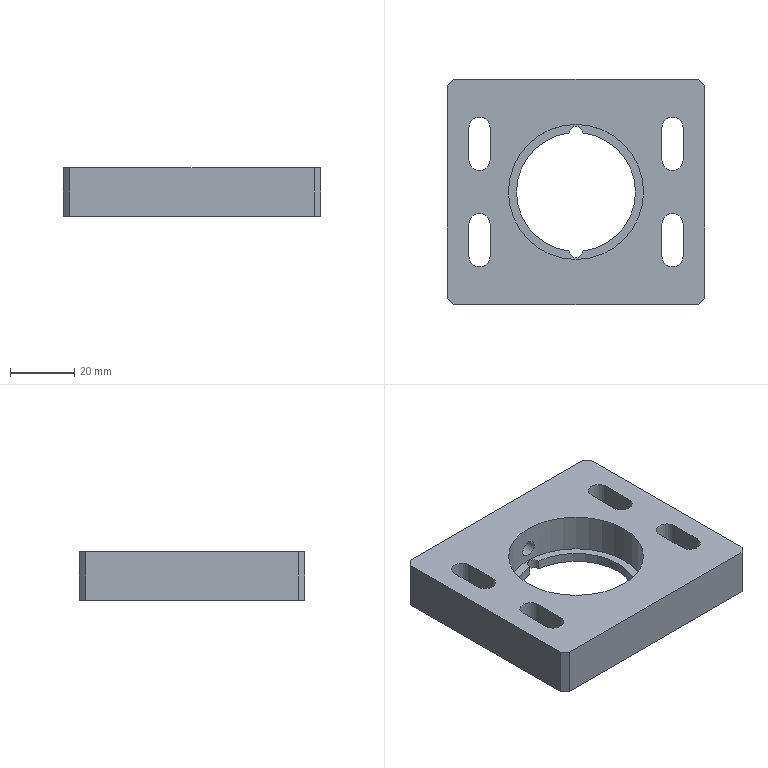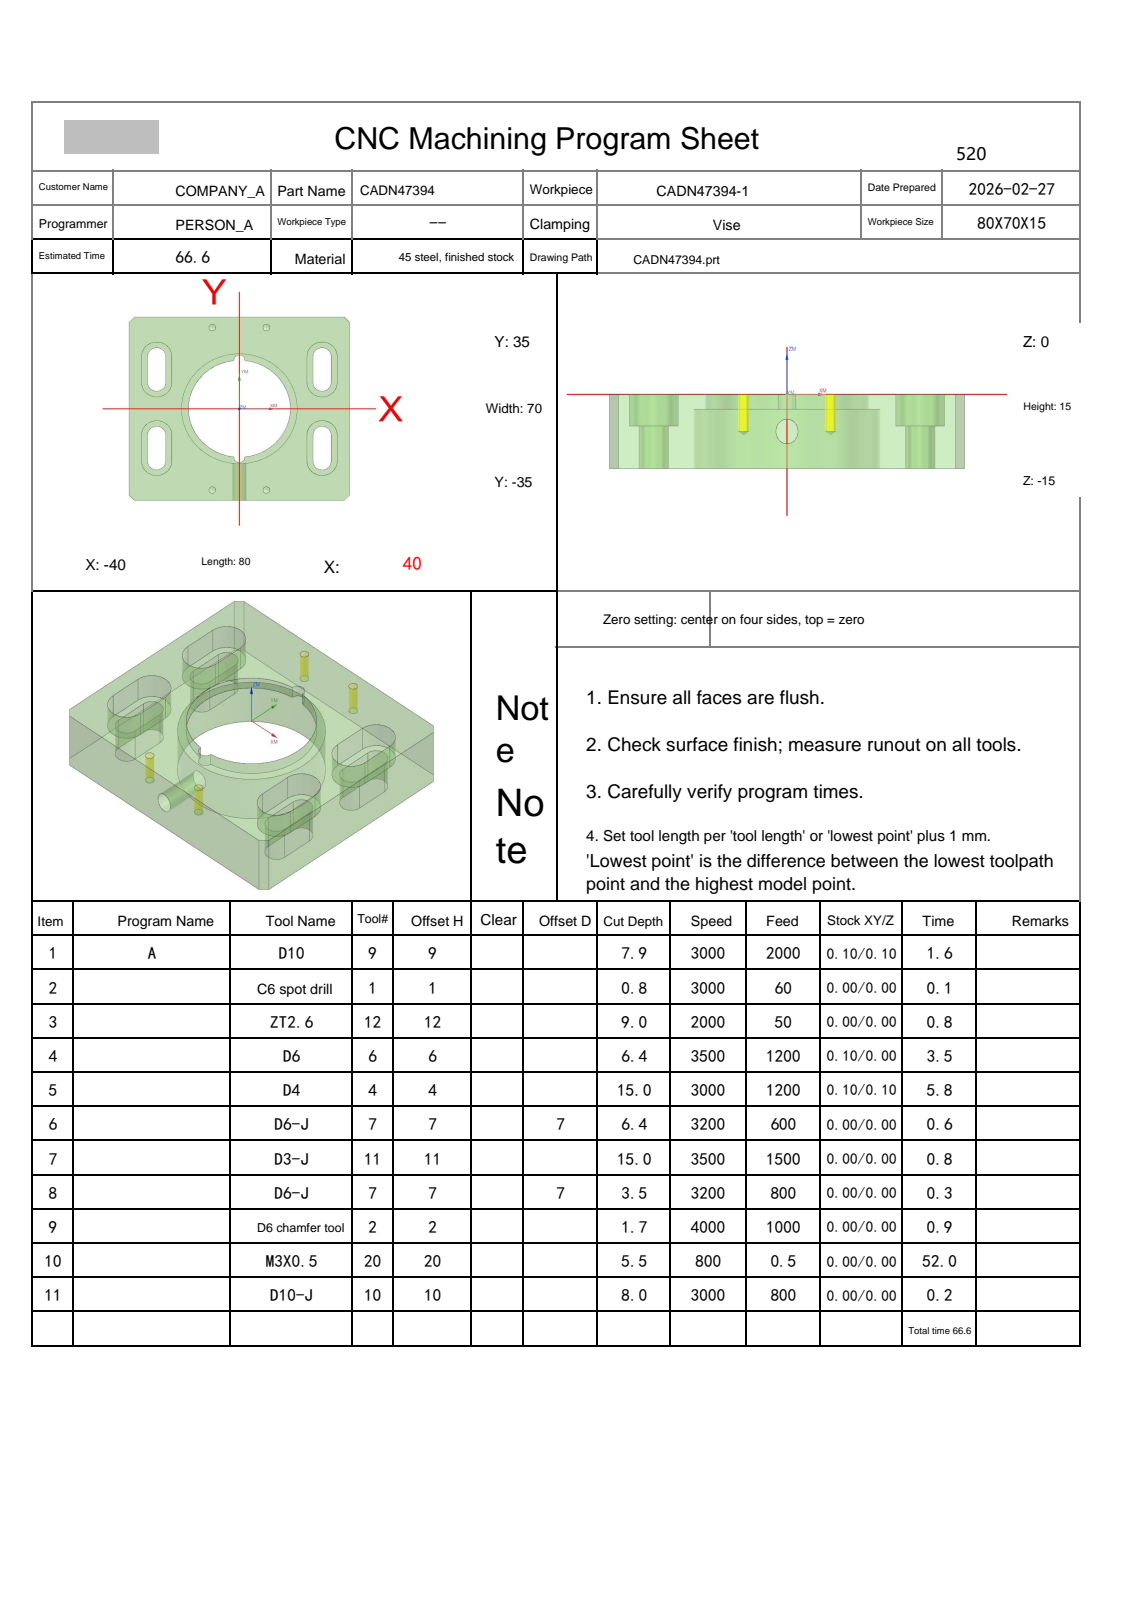NC program | NX | posted by the shop | part box 80 x 70 x 15 mm
Lines 1 to 1591 of 4817, first 1439 of 1589 lines:
%
O0001
(Machine time: 112.57 MIN)
(===Total Tool:10===)
(T9=D10     D=10.  R=0.   D-  H09 Z=-7.9  )
(T1=C6 spot drill   D=6.   R=0.   D-  H01 Z=-0.8  )
(T12=ZT2.6  D=2.6  DR_a=118 D-  H12 Z=-9.   )
(T6=D6      D=6.   R=0.   D-  H06 Z=-6.4  )
(T4=D4      D=4.   R=0.   D-  H04 Z=-15.  )
(T7=D6-J    D=6.   R=0.   D7  H07 Z=-6.4  )
(T11=D3-J   D=3.   R=0.   D11 H11 Z=-15.  )
(T2=D6 chamfer tool   D=6.   R=0.   D2  H02 Z=-1.75 )
(T20=M3X0.5 D=2.5  DR_a=180 D-  H20 Z=-5.5  )
(T10=D10-J  D=10.  R=0.   D-  H10 Z=-8.   )
G80 G90 G17 G49 G40
G91 G28 Z0
M01
N1 T09 M06
(D10  D=10. R=0. H=09 ce=0.10 di=0.10)
G00 G90 G54 X-35.242 Y-44.97 M03 S3000
G43 H09 Z50.
M08
Z-.5
G01 X-41.606 Y-38.606 F2000.
X-43.606 Y-36.606
X-49.97 Y-30.242
G00 Z-1.
G01 X-43.606 Y-36.606
X-41.606 Y-38.606
X-35.242 Y-44.97
G00 Z-1.5
G01 X-41.606 Y-38.606
X-43.606 Y-36.606
X-49.97 Y-30.242
G00 Z-2.
G01 X-43.606 Y-36.606
X-41.606 Y-38.606
X-35.242 Y-44.97
G00 Z-2.5
G01 X-41.606 Y-38.606
X-43.606 Y-36.606
X-49.97 Y-30.242
G00 Z-3.
G01 X-43.606 Y-36.606
X-41.606 Y-38.606
X-35.242 Y-44.97
G00 Z-3.5
G01 X-41.606 Y-38.606
X-43.606 Y-36.606
X-49.97 Y-30.242
G00 Z-4.
G01 X-43.606 Y-36.606
X-41.606 Y-38.606
X-35.242 Y-44.97
G00 Z-4.5
G01 X-41.606 Y-38.606
X-43.606 Y-36.606
X-49.97 Y-30.242
G00 Z-5.
G01 X-43.606 Y-36.606
X-41.606 Y-38.606
X-35.242 Y-44.97
G00 Z-5.5
G01 X-41.606 Y-38.606
X-43.606 Y-36.606
X-49.97 Y-30.242
G00 Z-6.
G01 X-43.606 Y-36.606
X-41.606 Y-38.606
X-35.242 Y-44.97
G00 Z-6.5
G01 X-41.606 Y-38.606
X-43.606 Y-36.606
X-49.97 Y-30.242
G00 Z-7.
G01 X-43.606 Y-36.606
X-41.606 Y-38.606
X-35.242 Y-44.97
G00 Z-7.5
G01 X-41.606 Y-38.606
X-43.606 Y-36.606
X-49.97 Y-30.242
G00 Z-7.9
G01 X-43.606 Y-36.606
X-41.606 Y-38.606
X-35.242 Y-44.97
G00 Z50.
X-49.97 Y30.242
Z-.5
G01 X-43.606 Y36.606
X-41.606 Y38.606
X-35.242 Y44.97
G00 Z-1.
G01 X-41.606 Y38.606
X-43.606 Y36.606
X-49.97 Y30.242
G00 Z-1.5
G01 X-43.606 Y36.606
X-41.606 Y38.606
X-35.242 Y44.97
G00 Z-2.
G01 X-41.606 Y38.606
X-43.606 Y36.606
X-49.97 Y30.242
G00 Z-2.5
G01 X-43.606 Y36.606
X-41.606 Y38.606
X-35.242 Y44.97
G00 Z-3.
G01 X-41.606 Y38.606
X-43.606 Y36.606
X-49.97 Y30.242
G00 Z-3.5
G01 X-43.606 Y36.606
X-41.606 Y38.606
X-35.242 Y44.97
G00 Z-4.
G01 X-41.606 Y38.606
X-43.606 Y36.606
X-49.97 Y30.242
G00 Z-4.5
G01 X-43.606 Y36.606
X-41.606 Y38.606
X-35.242 Y44.97
G00 Z-5.
G01 X-41.606 Y38.606
X-43.606 Y36.606
X-49.97 Y30.242
G00 Z-5.5
G01 X-43.606 Y36.606
X-41.606 Y38.606
X-35.242 Y44.97
G00 Z-6.
G01 X-41.606 Y38.606
X-43.606 Y36.606
X-49.97 Y30.242
G00 Z-6.5
G01 X-43.606 Y36.606
X-41.606 Y38.606
X-35.242 Y44.97
G00 Z-7.
G01 X-41.606 Y38.606
X-43.606 Y36.606
X-49.97 Y30.242
G00 Z-7.5
G01 X-43.606 Y36.606
X-41.606 Y38.606
X-35.242 Y44.97
G00 Z-7.9
G01 X-41.606 Y38.606
X-43.606 Y36.606
X-49.97 Y30.242
G00 Z50.
X35.242 Y44.97
Z-.5
G01 X41.606 Y38.606
X43.606 Y36.606
X49.97 Y30.242
G00 Z-1.
G01 X43.606 Y36.606
X41.606 Y38.606
X35.242 Y44.97
G00 Z-1.5
G01 X41.606 Y38.606
X43.606 Y36.606
X49.97 Y30.242
G00 Z-2.
G01 X43.606 Y36.606
X41.606 Y38.606
X35.242 Y44.97
G00 Z-2.5
G01 X41.606 Y38.606
X43.606 Y36.606
X49.97 Y30.242
G00 Z-3.
G01 X43.606 Y36.606
X41.606 Y38.606
X35.242 Y44.97
G00 Z-3.5
G01 X41.606 Y38.606
X43.606 Y36.606
X49.97 Y30.242
G00 Z-4.
G01 X43.606 Y36.606
X41.606 Y38.606
X35.242 Y44.97
G00 Z-4.5
G01 X41.606 Y38.606
X43.606 Y36.606
X49.97 Y30.242
G00 Z-5.
G01 X43.606 Y36.606
X41.606 Y38.606
X35.242 Y44.97
G00 Z-5.5
G01 X41.606 Y38.606
X43.606 Y36.606
X49.97 Y30.242
G00 Z-6.
G01 X43.606 Y36.606
X41.606 Y38.606
X35.242 Y44.97
G00 Z-6.5
G01 X41.606 Y38.606
X43.606 Y36.606
X49.97 Y30.242
G00 Z-7.
G01 X43.606 Y36.606
X41.606 Y38.606
X35.242 Y44.97
G00 Z-7.5
G01 X41.606 Y38.606
X43.606 Y36.606
X49.97 Y30.242
G00 Z-7.9
G01 X43.606 Y36.606
X41.606 Y38.606
X35.242 Y44.97
G00 Z50.
X49.97 Y-30.242
Z-.5
G01 X43.606 Y-36.606
X41.606 Y-38.606
X35.242 Y-44.97
G00 Z-1.
G01 X41.606 Y-38.606
X43.606 Y-36.606
X49.97 Y-30.242
G00 Z-1.5
G01 X43.606 Y-36.606
X41.606 Y-38.606
X35.242 Y-44.97
G00 Z-2.
G01 X41.606 Y-38.606
X43.606 Y-36.606
X49.97 Y-30.242
G00 Z-2.5
G01 X43.606 Y-36.606
X41.606 Y-38.606
X35.242 Y-44.97
G00 Z-3.
G01 X41.606 Y-38.606
X43.606 Y-36.606
X49.97 Y-30.242
G00 Z-3.5
G01 X43.606 Y-36.606
X41.606 Y-38.606
X35.242 Y-44.97
G00 Z-4.
G01 X41.606 Y-38.606
X43.606 Y-36.606
X49.97 Y-30.242
G00 Z-4.5
G01 X43.606 Y-36.606
X41.606 Y-38.606
X35.242 Y-44.97
G00 Z-5.
G01 X41.606 Y-38.606
X43.606 Y-36.606
X49.97 Y-30.242
G00 Z-5.5
G01 X43.606 Y-36.606
X41.606 Y-38.606
X35.242 Y-44.97
G00 Z-6.
G01 X41.606 Y-38.606
X43.606 Y-36.606
X49.97 Y-30.242
G00 Z-6.5
G01 X43.606 Y-36.606
X41.606 Y-38.606
X35.242 Y-44.97
G00 Z-7.
G01 X41.606 Y-38.606
X43.606 Y-36.606
X49.97 Y-30.242
G00 Z-7.5
G01 X43.606 Y-36.606
X41.606 Y-38.606
X35.242 Y-44.97
G00 Z-7.9
G01 X41.606 Y-38.606
X43.606 Y-36.606
X49.97 Y-30.242
G00 Z50.
G00 G90 X.03 Y3.929 M03 S3000
Z10.1
Z1.5
G02 X.03 Y3.929 Z.018 I2.973 J3.378 F2000.
X2.009 Y11.696 Z-.5 I2.973 J3.378
G01 X5.094 Y12.394
G02 X5.8 Y12.08 I-5.112 J-12.44
X13.4 Y0.0 I-5.8 J-12.08
X1.447 Y-13.322 I-13.4 J0.0
G03 X0.0 Y-13.699 I.551 J-5.07
X-1.447 Y-13.322 I-1.997 J-4.693
G02 X-13.4 Y0.0 I1.447 J13.322
X-5.8 Y12.08 I13.4 J0.0
X-4.37 Y12.667 I5.819 J-12.126
X-1.447 Y13.322 I4.37 J-12.667
G03 X0.0 Y13.699 I-.551 J5.07
X1.447 Y13.322 I1.997 J4.693
G02 X4.37 Y12.667 I-1.447 J-13.322
X5.8 Y12.08 I-4.389 J-12.714
X8.684 Y10.205 I-5.8 J-12.08
X9.036 Y9.444 I-.648 J-.761
X8.937 Y9.011 I-1. J0.0
G01 X6.043 Y2.991
G03 X5.944 Y2.558 I.901 J-.433
X6.005 Y2.212 I1. J0.0
G02 X6.4 Y0.0 I-6.005 J-2.212
X5.2 Y-3.731 I-6.4 J0.0
X.623 Y-6.37 I-5.201 J3.731
G03 X.152 Y-6.433 I1.374 J-12.022
G01 X0.0 Y-6.445
X-.152 Y-6.433
G03 X-.691 Y-6.363 I-1.845 J-11.958
G02 X-6.4 Y0.0 I.691 J6.363
X-2.771 Y5.769 I6.4 J0.0
X-2.087 Y6.05 I2.79 J-5.815
X-.623 Y6.37 I2.089 J-6.05
G03 X-.152 Y6.433 I-1.374 J12.022
G01 X0.0 Y6.445
X.152 Y6.433
G03 X.691 Y6.363 I1.845 J11.958
G02 X1.735 Y6.16 I-.691 J-6.363
X2.464 Y5.198 I-.271 J-.962
G01 X2.456 Y5.068
X1.87 Y.597
X1.862 Y.468
X1.875 Y.307
G02 X1.9 Y0.0 I-1.875 J-.307
X1.544 Y-1.108 I-1.9 J0.0
X.112 Y-1.899 I-1.547 J1.107
G01 X0.0 Y-1.906
X-.112 Y-1.899
X-.205 Y-1.889
G02 X-1.9 Y0.0 I.205 J1.889
X-.823 Y1.712 I1.9 J0.0
X-.618 Y1.797 I.842 J-1.758
X-.112 Y1.899 I.628 J-1.796
G01 X0.0 Y1.906
X.112 Y1.899
X.205 Y1.889
G02 X.618 Y1.797 I-.205 J-1.889
X.823 Y1.712 I-.637 J-1.843
X1.313 Y1.373 I-.823 J-1.712
X1.625 Y.984 I-1.313 J-1.373
G03 X7.613 Y-2.389 I5.987 J3.626
X11.239 Y-1.377 I0.0 J7.
G01 Z.7
G00 Z3.
G01 X.03 Y3.929 F6000.
G00 Z1.
G02 X.03 Y3.929 Z-.482 I2.973 J3.378 F2000.
X2.009 Y11.696 Z-1. I2.973 J3.378
G01 X5.094 Y12.394
G02 X5.8 Y12.08 I-5.112 J-12.44
X13.4 Y0.0 I-5.8 J-12.08
X1.447 Y-13.322 I-13.4 J0.0
G03 X0.0 Y-13.699 I.551 J-5.07
X-1.447 Y-13.322 I-1.997 J-4.693
G02 X-13.4 Y0.0 I1.447 J13.322
X-5.8 Y12.08 I13.4 J0.0
X-4.37 Y12.667 I5.819 J-12.126
X-1.447 Y13.322 I4.37 J-12.667
G03 X0.0 Y13.699 I-.551 J5.07
X1.447 Y13.322 I1.997 J4.693
G02 X4.37 Y12.667 I-1.447 J-13.322
X5.8 Y12.08 I-4.389 J-12.714
X8.684 Y10.205 I-5.8 J-12.08
X9.036 Y9.444 I-.648 J-.761
X8.937 Y9.011 I-1. J0.0
G01 X6.043 Y2.991
G03 X5.944 Y2.558 I.901 J-.433
X6.005 Y2.212 I1. J0.0
G02 X6.4 Y0.0 I-6.005 J-2.212
X5.2 Y-3.731 I-6.4 J0.0
X.623 Y-6.37 I-5.201 J3.731
G03 X.151 Y-6.434 I1.374 J-12.022
G01 X0.0 Y-6.445
X-.151 Y-6.434
G03 X-.691 Y-6.363 I-1.846 J-11.958
G02 X-6.4 Y0.0 I.691 J6.363
X-2.771 Y5.769 I6.4 J0.0
X-2.087 Y6.05 I2.79 J-5.815
X-1.426 Y6.239 I2.087 J-6.05
X-.623 Y6.37 I1.43 J-6.239
G03 X-.151 Y6.434 I-1.374 J12.022
G01 X0.0 Y6.445
X.151 Y6.434
G03 X.691 Y6.363 I1.846 J11.958
G02 X1.71 Y6.167 I-.691 J-6.363
X2.369 Y5.3 I-.241 J-.867
X2.336 Y5.06 I-.9 J0.0
G01 X1.452 Y1.872
G03 X1.415 Y1.605 I.964 J-.267
X1.582 Y1.052 I1. J0.0
G02 X1.9 Y0.0 I-1.582 J-1.052
X1.544 Y-1.108 I-1.9 J0.0
X.112 Y-1.899 I-1.547 J1.107
G01 X0.0 Y-1.906
X-.112 Y-1.899
G02 X-1.544 Y-1.108 I.114 J1.897
X-1.9 Y0.0 I1.544 J1.108
X-.823 Y1.712 I1.9 J0.0
X-.618 Y1.797 I.842 J-1.758
X-.423 Y1.852 I.618 J-1.797
X-.112 Y1.899 I.439 J-1.851
G01 X0.0 Y1.906
X.112 Y1.899
X.205 Y1.889
G02 X.619 Y1.797 I-.205 J-1.889
X.823 Y1.712 I-.637 J-1.843
X1.313 Y1.373 I-.823 J-1.712
X1.625 Y.984 I-1.313 J-1.373
G03 X7.613 Y-2.389 I5.987 J3.626
X11.239 Y-1.377 I0.0 J7.
G01 Z.2
G00 Z2.5
G01 X.03 Y3.929 F6000.
G00 Z.5
G02 X.03 Y3.929 Z-.982 I2.973 J3.378 F2000.
X2.009 Y11.696 Z-1.5 I2.973 J3.378
G01 X5.094 Y12.394
G02 X5.8 Y12.08 I-5.112 J-12.44
X13.4 Y0.0 I-5.8 J-12.08
X1.447 Y-13.322 I-13.4 J0.0
G03 X.373 Y-13.557 I.551 J-5.07
G01 X0.0 Y-13.699
G03 X-1.447 Y-13.322 I-1.997 J-4.693
G02 X-13.4 Y0.0 I1.447 J13.322
X-5.8 Y12.08 I13.4 J0.0
X-4.37 Y12.667 I5.819 J-12.126
X-1.447 Y13.322 I4.37 J-12.667
G03 X0.0 Y13.699 I-.551 J5.07
X1.447 Y13.322 I1.997 J4.693
G02 X4.37 Y12.667 I-1.447 J-13.322
X5.8 Y12.08 I-4.389 J-12.713
X8.684 Y10.205 I-5.8 J-12.08
X9.036 Y9.444 I-.648 J-.761
X8.937 Y9.011 I-1. J0.0
G01 X6.043 Y2.991
G03 X5.944 Y2.558 I.901 J-.433
X6.005 Y2.212 I1. J0.0
G02 X6.4 Y0.0 I-6.005 J-2.212
X5.2 Y-3.731 I-6.4 J0.0
X.623 Y-6.37 I-5.201 J3.731
G03 X.151 Y-6.434 I1.374 J-12.022
G01 X0.0 Y-6.445
X-.151 Y-6.434
G03 X-.691 Y-6.363 I-1.846 J-11.958
G02 X-6.4 Y0.0 I.691 J6.363
X-2.771 Y5.769 I6.4 J0.0
X-2.087 Y6.05 I2.79 J-5.815
X-.623 Y6.37 I2.089 J-6.05
G03 X-.151 Y6.434 I-1.374 J12.022
G01 X0.0 Y6.445
X.151 Y6.434
G03 X.691 Y6.363 I1.846 J11.958
G02 X1.71 Y6.167 I-.691 J-6.363
X2.369 Y5.3 I-.241 J-.867
X2.336 Y5.06 I-.9 J0.0
G01 X1.452 Y1.872
G03 X1.415 Y1.605 I.964 J-.267
X1.582 Y1.052 I1. J0.0
G02 X1.9 Y0.0 I-1.582 J-1.052
X1.544 Y-1.108 I-1.9 J0.0
X.112 Y-1.899 I-1.547 J1.107
G01 X0.0 Y-1.906
X-.112 Y-1.899
G02 X-1.544 Y-1.108 I.114 J1.897
X-1.9 Y0.0 I1.544 J1.108
X-.823 Y1.712 I1.9 J0.0
X-.618 Y1.797 I.842 J-1.758
X-.112 Y1.899 I.628 J-1.796
G01 X0.0 Y1.906
X.112 Y1.899
X.205 Y1.889
G02 X.619 Y1.797 I-.205 J-1.889
X.823 Y1.712 I-.637 J-1.843
X1.313 Y1.373 I-.823 J-1.712
X1.625 Y.984 I-1.313 J-1.373
G03 X7.613 Y-2.389 I5.987 J3.626
X11.239 Y-1.377 I0.0 J7.
G01 Z-.3
G00 Z2.
G01 X.03 Y3.929 F6000.
G00 Z0.0
G02 X.03 Y3.929 Z-1.482 I2.973 J3.378 F2000.
X2.009 Y11.696 Z-2. I2.973 J3.378
G01 X5.094 Y12.394
G02 X5.8 Y12.08 I-5.112 J-12.44
X13.4 Y0.0 I-5.8 J-12.08
X1.447 Y-13.322 I-13.4 J0.0
G03 X0.0 Y-13.699 I.551 J-5.07
X-1.447 Y-13.322 I-1.997 J-4.693
G02 X-13.4 Y0.0 I1.447 J13.322
X-5.8 Y12.08 I13.4 J0.0
X-4.37 Y12.667 I5.819 J-12.126
X-1.447 Y13.322 I4.37 J-12.667
G03 X0.0 Y13.699 I-.551 J5.07
X1.447 Y13.322 I1.997 J4.693
G02 X4.37 Y12.667 I-1.447 J-13.322
X5.8 Y12.08 I-4.389 J-12.713
X8.684 Y10.205 I-5.8 J-12.08
X9.036 Y9.444 I-.648 J-.761
X8.937 Y9.011 I-1. J0.0
G01 X6.043 Y2.991
G03 X5.944 Y2.558 I.901 J-.433
X6.005 Y2.212 I1. J0.0
G02 X6.4 Y0.0 I-6.005 J-2.212
X5.2 Y-3.731 I-6.4 J0.0
X.623 Y-6.37 I-5.201 J3.731
G03 X.151 Y-6.434 I1.374 J-12.022
G01 X0.0 Y-6.445
X-.151 Y-6.434
G03 X-.691 Y-6.363 I-1.846 J-11.958
G02 X-6.4 Y0.0 I.691 J6.363
X-2.771 Y5.769 I6.4 J0.0
X-2.087 Y6.05 I2.79 J-5.815
X-.623 Y6.37 I2.089 J-6.05
G03 X-.151 Y6.434 I-1.374 J12.022
G01 X0.0 Y6.445
X.151 Y6.434
G03 X.691 Y6.363 I1.846 J11.958
G02 X1.71 Y6.167 I-.691 J-6.363
X2.369 Y5.3 I-.241 J-.867
X2.336 Y5.06 I-.9 J0.0
G01 X1.452 Y1.872
G03 X1.415 Y1.605 I.964 J-.267
X1.582 Y1.052 I1. J0.0
G02 X1.9 Y0.0 I-1.582 J-1.052
X1.544 Y-1.108 I-1.9 J0.0
X.112 Y-1.899 I-1.547 J1.107
G01 X0.0 Y-1.906
X-.112 Y-1.899
G02 X-1.544 Y-1.108 I.114 J1.897
X-1.9 Y0.0 I1.544 J1.108
X-.823 Y1.712 I1.9 J0.0
X-.619 Y1.797 I.842 J-1.758
X-.112 Y1.899 I.628 J-1.796
G01 X0.0 Y1.906
X.112 Y1.899
X.205 Y1.889
G02 X.619 Y1.797 I-.205 J-1.889
X.823 Y1.712 I-.637 J-1.843
X1.313 Y1.373 I-.823 J-1.712
X1.625 Y.984 I-1.313 J-1.373
G03 X7.613 Y-2.389 I5.987 J3.626
X11.239 Y-1.377 I0.0 J7.
G01 Z-.8
G00 Z1.5
G01 X.03 Y3.929 F6000.
G00 Z-.5
G02 X.03 Y3.929 Z-1.982 I2.973 J3.378 F2000.
X2.009 Y11.696 Z-2.5 I2.973 J3.378
G01 X5.094 Y12.394
G02 X5.8 Y12.08 I-5.112 J-12.44
X13.4 Y0.0 I-5.8 J-12.08
X1.447 Y-13.322 I-13.4 J0.0
G03 X0.0 Y-13.699 I.551 J-5.07
X-1.447 Y-13.322 I-1.997 J-4.693
G02 X-13.4 Y0.0 I1.447 J13.322
X-5.8 Y12.08 I13.4 J0.0
X-4.37 Y12.667 I5.819 J-12.126
X-1.447 Y13.322 I4.37 J-12.667
G03 X0.0 Y13.699 I-.551 J5.07
X1.447 Y13.322 I1.997 J4.693
G02 X4.37 Y12.667 I-1.447 J-13.322
X5.8 Y12.08 I-4.389 J-12.713
X8.684 Y10.205 I-5.8 J-12.08
X9.036 Y9.444 I-.648 J-.761
X8.937 Y9.011 I-1. J0.0
G01 X6.043 Y2.991
G03 X5.944 Y2.558 I.901 J-.433
X6.005 Y2.212 I1. J0.0
G02 X6.4 Y0.0 I-6.005 J-2.212
X5.2 Y-3.731 I-6.4 J0.0
X.623 Y-6.37 I-5.201 J3.731
G03 X.151 Y-6.434 I1.374 J-12.022
G01 X0.0 Y-6.445
X-.151 Y-6.434
G03 X-.691 Y-6.363 I-1.846 J-11.958
G02 X-6.4 Y0.0 I.691 J6.363
X-2.771 Y5.769 I6.4 J0.0
X-2.087 Y6.05 I2.79 J-5.815
X-1.289 Y6.269 I2.087 J-6.05
X-.623 Y6.37 I1.294 J-6.268
G03 X-.151 Y6.434 I-1.374 J12.022
G01 X0.0 Y6.445
X.151 Y6.434
G03 X.691 Y6.363 I1.846 J11.958
G02 X1.71 Y6.167 I-.691 J-6.363
X2.369 Y5.3 I-.241 J-.867
X2.336 Y5.06 I-.9 J0.0
G01 X1.452 Y1.872
G03 X1.415 Y1.605 I.964 J-.267
X1.582 Y1.052 I1. J0.0
G02 X1.9 Y0.0 I-1.582 J-1.052
X1.544 Y-1.108 I-1.9 J0.0
X.112 Y-1.899 I-1.547 J1.107
G01 X0.0 Y-1.906
X-.112 Y-1.899
G02 X-1.544 Y-1.108 I.113 J1.897
X-1.9 Y0.0 I1.544 J1.108
X-.823 Y1.712 I1.9 J0.0
X-.619 Y1.797 I.842 J-1.758
X-.383 Y1.861 I.619 J-1.797
X-.111 Y1.899 I.401 J-1.86
G01 X0.0 Y1.906
X.112 Y1.899
X.205 Y1.889
G02 X.619 Y1.797 I-.205 J-1.889
X.823 Y1.712 I-.638 J-1.843
X1.313 Y1.373 I-.823 J-1.712
X1.625 Y.984 I-1.313 J-1.373
G03 X7.613 Y-2.389 I5.987 J3.626
X11.239 Y-1.377 I0.0 J7.
G01 Z-1.3
G00 Z1.
G01 X.03 Y3.929 F6000.
G00 Z-1.
G02 X.03 Y3.929 Z-2.482 I2.973 J3.378 F2000.
X2.009 Y11.696 Z-3. I2.973 J3.378
G01 X5.094 Y12.394
G02 X5.8 Y12.08 I-5.112 J-12.44
X13.4 Y0.0 I-5.8 J-12.08
X1.447 Y-13.322 I-13.4 J0.0
G03 X0.0 Y-13.699 I.551 J-5.07
X-1.447 Y-13.322 I-1.997 J-4.693
G02 X-13.4 Y0.0 I1.447 J13.322
X-5.8 Y12.08 I13.4 J0.0
X-4.37 Y12.667 I5.819 J-12.126
X-1.447 Y13.322 I4.37 J-12.667
G03 X0.0 Y13.699 I-.551 J5.07
X1.447 Y13.322 I1.997 J4.693
G02 X4.37 Y12.667 I-1.447 J-13.322
X5.8 Y12.08 I-4.389 J-12.713
X8.684 Y10.205 I-5.8 J-12.08
X9.036 Y9.444 I-.648 J-.761
X8.937 Y9.011 I-1. J0.0
G01 X6.043 Y2.991
G03 X5.944 Y2.558 I.901 J-.433
X6.005 Y2.212 I1. J0.0
G02 X6.4 Y0.0 I-6.005 J-2.212
X5.2 Y-3.731 I-6.4 J0.0
X.623 Y-6.37 I-5.201 J3.731
G03 X.15 Y-6.434 I1.375 J-12.022
G01 X0.0 Y-6.445
X-.15 Y-6.434
G03 X-.691 Y-6.363 I-1.847 J-11.958
G02 X-6.4 Y0.0 I.691 J6.363
X-2.771 Y5.769 I6.4 J0.0
X-2.087 Y6.05 I2.79 J-5.815
X-.623 Y6.37 I2.089 J-6.05
G03 X-.15 Y6.434 I-1.375 J12.022
G01 X0.0 Y6.445
X.15 Y6.434
G03 X.691 Y6.363 I1.847 J11.958
G02 X1.71 Y6.167 I-.691 J-6.363
X2.369 Y5.3 I-.241 J-.867
X2.336 Y5.06 I-.9 J0.0
G01 X1.452 Y1.872
G03 X1.415 Y1.605 I.964 J-.267
X1.582 Y1.052 I1. J0.0
G02 X1.9 Y0.0 I-1.582 J-1.052
X1.544 Y-1.108 I-1.9 J0.0
X.111 Y-1.899 I-1.547 J1.107
G01 X0.0 Y-1.906
X-.111 Y-1.899
G02 X-1.544 Y-1.108 I.113 J1.897
X-1.9 Y0.0 I1.544 J1.108
X-.823 Y1.712 I1.9 J0.0
X-.619 Y1.797 I.842 J-1.758
X-.111 Y1.899 I.628 J-1.796
G01 X0.0 Y1.906
X.111 Y1.899
X.205 Y1.889
G02 X.619 Y1.797 I-.205 J-1.889
X.823 Y1.712 I-.637 J-1.843
X1.313 Y1.373 I-.823 J-1.712
X1.625 Y.984 I-1.313 J-1.373
G03 X7.613 Y-2.389 I5.987 J3.626
X11.239 Y-1.377 I0.0 J7.
G01 Z-1.8
G00 Z.5
G01 X.03 Y3.929 F6000.
G00 Z-1.5
G02 X.03 Y3.929 Z-2.982 I2.973 J3.378 F2000.
X2.009 Y11.696 Z-3.5 I2.973 J3.378
G01 X5.094 Y12.394
G02 X5.8 Y12.08 I-5.112 J-12.44
X13.4 Y0.0 I-5.8 J-12.08
X1.447 Y-13.322 I-13.4 J0.0
G03 X0.0 Y-13.699 I.551 J-5.07
X-1.447 Y-13.322 I-1.997 J-4.693
G02 X-13.4 Y0.0 I1.447 J13.322
X-5.8 Y12.08 I13.4 J0.0
X-4.37 Y12.667 I5.819 J-12.126
X-1.447 Y13.322 I4.37 J-12.667
G03 X0.0 Y13.699 I-.551 J5.07
X1.447 Y13.322 I1.997 J4.693
G02 X4.37 Y12.667 I-1.447 J-13.322
X5.8 Y12.08 I-4.389 J-12.713
X8.684 Y10.205 I-5.8 J-12.08
X9.036 Y9.444 I-.648 J-.761
X8.937 Y9.011 I-1. J0.0
G01 X6.043 Y2.991
G03 X5.944 Y2.558 I.901 J-.433
X6.005 Y2.212 I1. J0.0
G02 X6.4 Y0.0 I-6.005 J-2.212
X5.2 Y-3.731 I-6.4 J0.0
X.622 Y-6.37 I-5.201 J3.731
G03 X.15 Y-6.434 I1.375 J-12.022
G01 X0.0 Y-6.445
X-.15 Y-6.434
G03 X-.691 Y-6.363 I-1.847 J-11.958
G02 X-6.4 Y0.0 I.691 J6.363
X-2.771 Y5.769 I6.4 J0.0
X-2.087 Y6.05 I2.79 J-5.815
X-.622 Y6.37 I2.089 J-6.05
G03 X-.15 Y6.434 I-1.375 J12.022
G01 X0.0 Y6.445
X.15 Y6.434
G03 X.691 Y6.363 I1.847 J11.958
G02 X1.71 Y6.167 I-.691 J-6.363
X2.369 Y5.3 I-.241 J-.867
X2.336 Y5.06 I-.9 J0.0
G01 X1.452 Y1.872
G03 X1.415 Y1.605 I.964 J-.267
X1.582 Y1.052 I1. J0.0
G02 X1.9 Y0.0 I-1.582 J-1.052
X1.544 Y-1.108 I-1.9 J0.0
X.111 Y-1.899 I-1.547 J1.107
G01 X0.0 Y-1.906
X-.111 Y-1.899
G02 X-1.544 Y-1.108 I.113 J1.897
X-1.9 Y0.0 I1.544 J1.108
X-.823 Y1.712 I1.9 J0.0
X-.619 Y1.797 I.842 J-1.758
X-.111 Y1.899 I.628 J-1.796
G01 X0.0 Y1.906
X.111 Y1.899
X.205 Y1.889
G02 X.619 Y1.797 I-.205 J-1.889
X.823 Y1.712 I-.638 J-1.843
X1.313 Y1.373 I-.823 J-1.712
X1.625 Y.984 I-1.313 J-1.373
G03 X7.613 Y-2.389 I5.987 J3.626
X11.239 Y-1.377 I0.0 J7.
G01 Z-2.3
G00 Z0.0
G01 X.03 Y3.929 F6000.
G00 Z-2.
G02 X.03 Y3.929 Z-3.482 I2.973 J3.378 F2000.
X2.009 Y11.696 Z-4. I2.973 J3.378
G01 X5.094 Y12.394
G02 X5.8 Y12.08 I-5.112 J-12.44
X13.4 Y0.0 I-5.8 J-12.08
X1.447 Y-13.322 I-13.4 J0.0
G03 X0.0 Y-13.699 I.551 J-5.07
X-1.447 Y-13.322 I-1.997 J-4.693
G02 X-13.4 Y0.0 I1.447 J13.322
X-5.8 Y12.08 I13.4 J0.0
X-4.37 Y12.667 I5.819 J-12.126
X-1.447 Y13.322 I4.37 J-12.667
G03 X0.0 Y13.699 I-.551 J5.07
X1.447 Y13.322 I1.997 J4.693
G02 X4.37 Y12.667 I-1.447 J-13.322
X5.8 Y12.08 I-4.389 J-12.713
X9.261 Y9.685 I-5.8 J-12.08
X9.57 Y8.962 I-.691 J-.723
X9.423 Y8.441 I-1. J0.0
G01 X6.112 Y3.019
G03 X5.965 Y2.498 I.854 J-.521
X6.024 Y2.161 I1. J0.0
G02 X6.4 Y0.0 I-6.024 J-2.161
X5.2 Y-3.731 I-6.4 J0.0
X.622 Y-6.37 I-5.201 J3.731
G03 X.15 Y-6.434 I1.375 J-12.022
G01 X0.0 Y-6.445
X-.15 Y-6.434
G03 X-.691 Y-6.363 I-1.847 J-11.958
G02 X-6.4 Y0.0 I.691 J6.363
X-2.771 Y5.769 I6.4 J0.0
X-2.087 Y6.05 I2.79 J-5.815
X-.622 Y6.37 I2.089 J-6.05
G03 X-.15 Y6.434 I-1.375 J12.022
G01 X0.0 Y6.445
X.15 Y6.434
G03 X.691 Y6.363 I1.847 J11.958
G02 X1.71 Y6.167 I-.691 J-6.363
X2.369 Y5.3 I-.241 J-.867
X2.336 Y5.06 I-.9 J0.0
G01 X1.452 Y1.872
G03 X1.415 Y1.605 I.964 J-.267
X1.582 Y1.052 I1. J0.0
G02 X1.9 Y0.0 I-1.582 J-1.052
X1.544 Y-1.108 I-1.9 J0.0
X.111 Y-1.899 I-1.547 J1.107
G01 X0.0 Y-1.906
X-.111 Y-1.899
G02 X-1.544 Y-1.108 I.113 J1.897
X-1.9 Y0.0 I1.544 J1.108
X-.823 Y1.712 I1.9 J0.0
X-.619 Y1.797 I.842 J-1.758
X-.111 Y1.899 I.628 J-1.796
G01 X0.0 Y1.906
X.111 Y1.899
X.205 Y1.889
G02 X.619 Y1.797 I-.205 J-1.889
X.823 Y1.712 I-.638 J-1.843
X1.313 Y1.373 I-.823 J-1.712
X1.625 Y.984 I-1.313 J-1.373
G03 X7.613 Y-2.389 I5.987 J3.626
X11.239 Y-1.377 I0.0 J7.
G01 Z-2.8
G00 Z10.1
G91 G28 Z0.0
M05
M09
G91 G28 Z0.0
M01
N2 T01 M06
(C6 spot drill  D=6. R=0. H=01 ce=0.00 di=0.10)
G00 G90 G54 X9.8 Y-31. M03 S3000
G43 H01 Z50.
M08
G98 G81 X9.8 Y-31. Z-.8 R1. F60.
X-9.8
Y31.
X9.8
G80
G00 Z50.
G91 G28 Z0.0
M05
M09
G91 G28 Z0.0
M01
N3 T12 M06
(ZT2.6 D=2.6 DR_a=118 H=12)
G00 G90 G54 X9.8 Y-31. M03 S2000
G43 H12 Z50.
M08
G98 G83 X9.8 Y-31. Z-9. R1. F50. Q1.
X-9.8
Y31.
X9.8
G80
G00 Z50.
G91 G28 Z0.0
M05
M09
G91 G28 Z0.0
M01
N4 T06 M06
(D6  D=6. R=0. H=06 ce=0.10 di=0.00)
G00 G90 G54 X-32.4 Y15. M03 S3500
G43 H06 Z50.
M08
Z.5
G01 Y10. Z.465 F1200.
G03 X-30. Y7.6 Z.438 I2.4 J0.0
X-27.6 Y10. Z.412 I0.0 J2.4
G01 Y20. Z.342
G03 X-30. Y22.4 Z.315 I-2.4 J0.0
X-32.4 Y20. Z.289 I0.0 J-2.4
G01 Y10. Z.218
G03 X-30. Y7.6 Z.192 I2.4 J0.0
X-27.6 Y10. Z.165 I0.0 J2.4
G01 Y20. Z.095
G03 X-30. Y22.4 Z.069 I-2.4 J0.0
X-32.4 Y20. Z.042 I0.0 J-2.4
G01 Y10. Z-.028
G03 X-30. Y7.6 Z-.054 I2.4 J0.0
X-27.6 Y10. Z-.081 I0.0 J2.4
G01 Y20. Z-.151
G03 X-30. Y22.4 Z-.178 I-2.4 J0.0
X-32.4 Y20. Z-.204 I0.0 J-2.4
G01 Y10. Z-.274
G03 X-30. Y7.6 Z-.301 I2.4 J0.0
X-27.6 Y10. Z-.327 I0.0 J2.4
G01 Y20. Z-.398
G03 X-30. Y22.4 Z-.424 I-2.4 J0.0
X-32.4 Y20. Z-.451 I0.0 J-2.4
G01 Y10. Z-.521
G03 X-30. Y7.6 Z-.547 I2.4 J0.0
X-27.6 Y10. Z-.574 I0.0 J2.4
G01 Y20. Z-.644
G03 X-30. Y22.4 Z-.671 I-2.4 J0.0
X-32.4 Y20. Z-.697 I0.0 J-2.4
G01 Y10. Z-.767
G03 X-30. Y7.6 Z-.794 I2.4 J0.0
X-27.6 Y10. Z-.82 I0.0 J2.4
G01 Y20. Z-.89
G03 X-30. Y22.4 Z-.917 I-2.4 J0.0
X-32.4 Y20. Z-.943 I0.0 J-2.4
G01 Y10. Z-1.014
G03 X-30. Y7.6 Z-1.04 I2.4 J0.0
X-27.6 Y10. Z-1.067 I0.0 J2.4
G01 Y20. Z-1.137
G03 X-30. Y22.4 Z-1.163 I-2.4 J0.0
X-32.4 Y20. Z-1.19 I0.0 J-2.4
G01 Y10. Z-1.26
G03 X-30. Y7.6 Z-1.287 I2.4 J0.0
X-27.6 Y10. Z-1.313 I0.0 J2.4
G01 Y20. Z-1.383
G03 X-30. Y22.4 Z-1.41 I-2.4 J0.0
X-32.4 Y20. Z-1.436 I0.0 J-2.4
G01 Y10. Z-1.507
G03 X-30. Y7.6 Z-1.533 I2.4 J0.0
X-27.6 Y10. Z-1.56 I0.0 J2.4
G01 Y20. Z-1.63
G03 X-30. Y22.4 Z-1.656 I-2.4 J0.0
X-32.4 Y20. Z-1.683 I0.0 J-2.4
G01 Y10. Z-1.753
G03 X-30. Y7.6 Z-1.779 I2.4 J0.0
X-27.6 Y10. Z-1.806 I0.0 J2.4
G01 Y20. Z-1.876
G03 X-30. Y22.4 Z-1.903 I-2.4 J0.0
X-32.4 Y20. Z-1.929 I0.0 J-2.4
G01 Y10. Z-1.999
G03 X-30. Y7.6 Z-2.026 I2.4 J0.0
X-27.6 Y10. Z-2.052 I0.0 J2.4
G01 Y20. Z-2.123
G03 X-30. Y22.4 Z-2.149 I-2.4 J0.0
X-32.4 Y20. Z-2.176 I0.0 J-2.4
G01 Y10. Z-2.246
G03 X-30. Y7.6 Z-2.272 I2.4 J0.0
X-27.6 Y10. Z-2.299 I0.0 J2.4
G01 Y20. Z-2.369
G03 X-30. Y22.4 Z-2.396 I-2.4 J0.0
X-32.4 Y20. Z-2.422 I0.0 J-2.4
G01 Y10. Z-2.492
G03 X-30. Y7.6 Z-2.519 I2.4 J0.0
X-27.6 Y10. Z-2.545 I0.0 J2.4
G01 Y20. Z-2.615
G03 X-30. Y22.4 Z-2.642 I-2.4 J0.0
X-32.4 Y20. Z-2.668 I0.0 J-2.4
G01 Y10. Z-2.739
G03 X-30. Y7.6 Z-2.765 I2.4 J0.0
X-27.6 Y10. Z-2.792 I0.0 J2.4
G01 Y20. Z-2.862
G03 X-30. Y22.4 Z-2.888 I-2.4 J0.0
X-32.4 Y20. Z-2.915 I0.0 J-2.4
G01 Y10. Z-2.985
G03 X-30. Y7.6 Z-3.012 I2.4 J0.0
X-27.6 Y10. Z-3.038 I0.0 J2.4
G01 Y20. Z-3.108
G03 X-30. Y22.4 Z-3.135 I-2.4 J0.0
X-32.4 Y20. Z-3.161 I0.0 J-2.4
G01 Y10. Z-3.232
G03 X-30. Y7.6 Z-3.258 I2.4 J0.0
X-27.6 Y10. Z-3.285 I0.0 J2.4
G01 Y20. Z-3.355
G03 X-30. Y22.4 Z-3.381 I-2.4 J0.0
X-32.4 Y20. Z-3.408 I0.0 J-2.4
G01 Y10. Z-3.478
G03 X-30. Y7.6 Z-3.504 I2.4 J0.0
X-27.6 Y10. Z-3.531 I0.0 J2.4
G01 Y20. Z-3.601
G03 X-30. Y22.4 Z-3.628 I-2.4 J0.0
X-32.4 Y20. Z-3.654 I0.0 J-2.4
G01 Y10. Z-3.724
G03 X-30. Y7.6 Z-3.751 I2.4 J0.0
X-27.6 Y10. Z-3.777 I0.0 J2.4
G01 Y20. Z-3.848
G03 X-30. Y22.4 Z-3.874 I-2.4 J0.0
X-32.4 Y20. Z-3.901 I0.0 J-2.4
G01 Y10. Z-3.971
G03 X-30. Y7.6 Z-3.997 I2.4 J0.0
X-27.6 Y10. Z-4.024 I0.0 J2.4
G01 Y20. Z-4.094
G03 X-30. Y22.4 Z-4.121 I-2.4 J0.0
X-32.4 Y20. Z-4.147 I0.0 J-2.4
G01 Y10. Z-4.217
G03 X-30. Y7.6 Z-4.244 I2.4 J0.0
X-27.6 Y10. Z-4.27 I0.0 J2.4
G01 Y20. Z-4.34
G03 X-30. Y22.4 Z-4.367 I-2.4 J0.0
X-32.4 Y20. Z-4.393 I0.0 J-2.4
G01 Y10. Z-4.464
G03 X-30. Y7.6 Z-4.49 I2.4 J0.0
X-27.6 Y10. Z-4.517 I0.0 J2.4
G01 Y20. Z-4.587
G03 X-30. Y22.4 Z-4.613 I-2.4 J0.0
X-32.4 Y20. Z-4.64 I0.0 J-2.4
G01 Y10. Z-4.71
G03 X-30. Y7.6 Z-4.737 I2.4 J0.0
X-27.6 Y10. Z-4.763 I0.0 J2.4
G01 Y20. Z-4.833
G03 X-30. Y22.4 Z-4.86 I-2.4 J0.0
X-32.4 Y20. Z-4.886 I0.0 J-2.4
G01 Y10. Z-4.957
G03 X-30. Y7.6 Z-4.983 I2.4 J0.0
X-27.6 Y10. Z-5.01 I0.0 J2.4
G01 Y20. Z-5.08
G03 X-30. Y22.4 Z-5.106 I-2.4 J0.0
X-32.4 Y20. Z-5.133 I0.0 J-2.4
G01 Y10. Z-5.203
G03 X-30. Y7.6 Z-5.229 I2.4 J0.0
X-27.6 Y10. Z-5.256 I0.0 J2.4
G01 Y20. Z-5.326
G03 X-30. Y22.4 Z-5.353 I-2.4 J0.0
X-32.4 Y20. Z-5.379 I0.0 J-2.4
G01 Y10. Z-5.449
G03 X-30. Y7.6 Z-5.476 I2.4 J0.0
X-27.6 Y10. Z-5.502 I0.0 J2.4
G01 Y20. Z-5.573
G03 X-30. Y22.4 Z-5.599 I-2.4 J0.0
X-32.4 Y20. Z-5.626 I0.0 J-2.4
G01 Y10. Z-5.696
G03 X-30. Y7.6 Z-5.722 I2.4 J0.0
X-27.6 Y10. Z-5.749 I0.0 J2.4
G01 Y20. Z-5.819
G03 X-30. Y22.4 Z-5.846 I-2.4 J0.0
X-32.4 Y20. Z-5.872 I0.0 J-2.4
G01 Y10. Z-5.942
G03 X-30. Y7.6 Z-5.969 I2.4 J0.0
X-27.6 Y10. Z-5.995 I0.0 J2.4
G01 Y20. Z-6.065
G03 X-30. Y22.4 Z-6.092 I-2.4 J0.0
X-32.4 Y20. Z-6.118 I0.0 J-2.4
G01 Y10. Z-6.189
G03 X-30. Y7.6 Z-6.215 I2.4 J0.0
X-27.6 Y10. Z-6.242 I0.0 J2.4
G01 Y20. Z-6.312
G03 X-30. Y22.4 Z-6.338 I-2.4 J0.0
X-32.4 Y20. Z-6.365 I0.0 J-2.4
G01 Y15. Z-6.4
Y10.
G03 X-30. Y7.6 I2.4 J0.0
X-27.6 Y10. I0.0 J2.4
G01 Y20.
G03 X-30. Y22.4 I-2.4 J0.0
X-32.4 Y20. I0.0 J-2.4
G01 Y15.
Y14.5
Z-5.4
G00 Z50.
Y-15.
Z.5
G01 Y-20. Z.465
G03 X-30. Y-22.4 Z.438 I2.4 J0.0
X-27.6 Y-20. Z.412 I0.0 J2.4
G01 Y-10. Z.342
G03 X-30. Y-7.6 Z.315 I-2.4 J0.0
X-32.4 Y-10. Z.289 I0.0 J-2.4
G01 Y-20. Z.218
G03 X-30. Y-22.4 Z.192 I2.4 J0.0
X-27.6 Y-20. Z.165 I0.0 J2.4
G01 Y-10. Z.095
G03 X-30. Y-7.6 Z.069 I-2.4 J0.0
X-32.4 Y-10. Z.042 I0.0 J-2.4
G01 Y-20. Z-.028
G03 X-30. Y-22.4 Z-.054 I2.4 J0.0
X-27.6 Y-20. Z-.081 I0.0 J2.4
G01 Y-10. Z-.151
G03 X-30. Y-7.6 Z-.178 I-2.4 J0.0
X-32.4 Y-10. Z-.204 I0.0 J-2.4
G01 Y-20. Z-.274
G03 X-30. Y-22.4 Z-.301 I2.4 J0.0
X-27.6 Y-20. Z-.327 I0.0 J2.4
G01 Y-10. Z-.398
G03 X-30. Y-7.6 Z-.424 I-2.4 J0.0
X-32.4 Y-10. Z-.451 I0.0 J-2.4
G01 Y-20. Z-.521
G03 X-30. Y-22.4 Z-.547 I2.4 J0.0
X-27.6 Y-20. Z-.574 I0.0 J2.4
G01 Y-10. Z-.644
G03 X-30. Y-7.6 Z-.671 I-2.4 J0.0
X-32.4 Y-10. Z-.697 I0.0 J-2.4
G01 Y-20. Z-.767
G03 X-30. Y-22.4 Z-.794 I2.4 J0.0
X-27.6 Y-20. Z-.82 I0.0 J2.4
G01 Y-10. Z-.89
G03 X-30. Y-7.6 Z-.917 I-2.4 J0.0
X-32.4 Y-10. Z-.943 I0.0 J-2.4
G01 Y-20. Z-1.014
G03 X-30. Y-22.4 Z-1.04 I2.4 J0.0
X-27.6 Y-20. Z-1.067 I0.0 J2.4
G01 Y-10. Z-1.137
G03 X-30. Y-7.6 Z-1.163 I-2.4 J0.0
X-32.4 Y-10. Z-1.19 I0.0 J-2.4
G01 Y-20. Z-1.26
G03 X-30. Y-22.4 Z-1.287 I2.4 J0.0
X-27.6 Y-20. Z-1.313 I0.0 J2.4
G01 Y-10. Z-1.383
G03 X-30. Y-7.6 Z-1.41 I-2.4 J0.0
X-32.4 Y-10. Z-1.436 I0.0 J-2.4
G01 Y-20. Z-1.507
G03 X-30. Y-22.4 Z-1.533 I2.4 J0.0
X-27.6 Y-20. Z-1.56 I0.0 J2.4
G01 Y-10. Z-1.63
G03 X-30. Y-7.6 Z-1.656 I-2.4 J0.0
X-32.4 Y-10. Z-1.683 I0.0 J-2.4
G01 Y-20. Z-1.753
G03 X-30. Y-22.4 Z-1.779 I2.4 J0.0
X-27.6 Y-20. Z-1.806 I0.0 J2.4
G01 Y-10. Z-1.876
G03 X-30. Y-7.6 Z-1.903 I-2.4 J0.0
X-32.4 Y-10. Z-1.929 I0.0 J-2.4
G01 Y-20. Z-1.999
G03 X-30. Y-22.4 Z-2.026 I2.4 J0.0
X-27.6 Y-20. Z-2.052 I0.0 J2.4
G01 Y-10. Z-2.123
G03 X-30. Y-7.6 Z-2.149 I-2.4 J0.0
X-32.4 Y-10. Z-2.176 I0.0 J-2.4
G01 Y-20. Z-2.246
G03 X-30. Y-22.4 Z-2.272 I2.4 J0.0
X-27.6 Y-20. Z-2.299 I0.0 J2.4
G01 Y-10. Z-2.369
G03 X-30. Y-7.6 Z-2.396 I-2.4 J0.0
X-32.4 Y-10. Z-2.422 I0.0 J-2.4
G01 Y-20. Z-2.492
G03 X-30. Y-22.4 Z-2.519 I2.4 J0.0
X-27.6 Y-20. Z-2.545 I0.0 J2.4
G01 Y-10. Z-2.615
G03 X-30. Y-7.6 Z-2.642 I-2.4 J0.0
X-32.4 Y-10. Z-2.668 I0.0 J-2.4
G01 Y-20. Z-2.739
G03 X-30. Y-22.4 Z-2.765 I2.4 J0.0
X-27.6 Y-20. Z-2.792 I0.0 J2.4
G01 Y-10. Z-2.862
G03 X-30. Y-7.6 Z-2.888 I-2.4 J0.0
X-32.4 Y-10. Z-2.915 I0.0 J-2.4
G01 Y-20. Z-2.985
G03 X-30. Y-22.4 Z-3.012 I2.4 J0.0
X-27.6 Y-20. Z-3.038 I0.0 J2.4
G01 Y-10. Z-3.108
G03 X-30. Y-7.6 Z-3.135 I-2.4 J0.0
X-32.4 Y-10. Z-3.161 I0.0 J-2.4
G01 Y-20. Z-3.232
G03 X-30. Y-22.4 Z-3.258 I2.4 J0.0
X-27.6 Y-20. Z-3.285 I0.0 J2.4
G01 Y-10. Z-3.355
G03 X-30. Y-7.6 Z-3.381 I-2.4 J0.0
X-32.4 Y-10. Z-3.408 I0.0 J-2.4
G01 Y-20. Z-3.478
G03 X-30. Y-22.4 Z-3.504 I2.4 J0.0
X-27.6 Y-20. Z-3.531 I0.0 J2.4
G01 Y-10. Z-3.601
G03 X-30. Y-7.6 Z-3.628 I-2.4 J0.0
X-32.4 Y-10. Z-3.654 I0.0 J-2.4
G01 Y-20. Z-3.724
G03 X-30. Y-22.4 Z-3.751 I2.4 J0.0
X-27.6 Y-20. Z-3.777 I0.0 J2.4
G01 Y-10. Z-3.848
G03 X-30. Y-7.6 Z-3.874 I-2.4 J0.0
X-32.4 Y-10. Z-3.901 I0.0 J-2.4
G01 Y-20. Z-3.971
G03 X-30. Y-22.4 Z-3.997 I2.4 J0.0
X-27.6 Y-20. Z-4.024 I0.0 J2.4
G01 Y-10. Z-4.094
G03 X-30. Y-7.6 Z-4.121 I-2.4 J0.0
X-32.4 Y-10. Z-4.147 I0.0 J-2.4
G01 Y-20. Z-4.217
G03 X-30. Y-22.4 Z-4.244 I2.4 J0.0
X-27.6 Y-20. Z-4.27 I0.0 J2.4
G01 Y-10. Z-4.34
G03 X-30. Y-7.6 Z-4.367 I-2.4 J0.0
X-32.4 Y-10. Z-4.393 I0.0 J-2.4
G01 Y-20. Z-4.464
G03 X-30. Y-22.4 Z-4.49 I2.4 J0.0
X-27.6 Y-20. Z-4.517 I0.0 J2.4
G01 Y-10. Z-4.587
G03 X-30. Y-7.6 Z-4.613 I-2.4 J0.0
X-32.4 Y-10. Z-4.64 I0.0 J-2.4
G01 Y-20. Z-4.71
G03 X-30. Y-22.4 Z-4.737 I2.4 J0.0
X-27.6 Y-20. Z-4.763 I0.0 J2.4
G01 Y-10. Z-4.833
G03 X-30. Y-7.6 Z-4.86 I-2.4 J0.0
X-32.4 Y-10. Z-4.886 I0.0 J-2.4
G01 Y-20. Z-4.957
G03 X-30. Y-22.4 Z-4.983 I2.4 J0.0
X-27.6 Y-20. Z-5.01 I0.0 J2.4
G01 Y-10. Z-5.08
G03 X-30. Y-7.6 Z-5.106 I-2.4 J0.0
X-32.4 Y-10. Z-5.133 I0.0 J-2.4
G01 Y-20. Z-5.203
G03 X-30. Y-22.4 Z-5.229 I2.4 J0.0
X-27.6 Y-20. Z-5.256 I0.0 J2.4
G01 Y-10. Z-5.326
G03 X-30. Y-7.6 Z-5.353 I-2.4 J0.0
X-32.4 Y-10. Z-5.379 I0.0 J-2.4
G01 Y-20. Z-5.449
G03 X-30. Y-22.4 Z-5.476 I2.4 J0.0
X-27.6 Y-20. Z-5.502 I0.0 J2.4
G01 Y-10. Z-5.573
G03 X-30. Y-7.6 Z-5.599 I-2.4 J0.0
X-32.4 Y-10. Z-5.626 I0.0 J-2.4
G01 Y-20. Z-5.696
G03 X-30. Y-22.4 Z-5.722 I2.4 J0.0
X-27.6 Y-20. Z-5.749 I0.0 J2.4
G01 Y-10. Z-5.819
G03 X-30. Y-7.6 Z-5.846 I-2.4 J0.0
X-32.4 Y-10. Z-5.872 I0.0 J-2.4
G01 Y-20. Z-5.942
G03 X-30. Y-22.4 Z-5.969 I2.4 J0.0
X-27.6 Y-20. Z-5.995 I0.0 J2.4
G01 Y-10. Z-6.065
G03 X-30. Y-7.6 Z-6.092 I-2.4 J0.0
X-32.4 Y-10. Z-6.118 I0.0 J-2.4
G01 Y-20. Z-6.189
G03 X-30. Y-22.4 Z-6.215 I2.4 J0.0
X-27.6 Y-20. Z-6.242 I0.0 J2.4
G01 Y-10. Z-6.312
G03 X-30. Y-7.6 Z-6.338 I-2.4 J0.0
X-32.4 Y-10. Z-6.365 I0.0 J-2.4
G01 Y-15. Z-6.4
Y-20.
G03 X-30. Y-22.4 I2.4 J0.0
X-27.6 Y-20. I0.0 J2.4
G01 Y-10.
G03 X-30. Y-7.6 I-2.4 J0.0
X-32.4 Y-10. I0.0 J-2.4
G01 Y-15.
Y-15.5
Z-5.4
G00 Z50.
X32.4 Y15.
Z.5
G01 Y20. Z.465
G03 X30. Y22.4 Z.438 I-2.4 J0.0
X27.6 Y20. Z.412 I0.0 J-2.4
G01 Y10. Z.342
G03 X30. Y7.6 Z.315 I2.4 J0.0
X32.4 Y10. Z.289 I0.0 J2.4
G01 Y20. Z.218
G03 X30. Y22.4 Z.192 I-2.4 J0.0
X27.6 Y20. Z.165 I0.0 J-2.4
G01 Y10. Z.095
G03 X30. Y7.6 Z.069 I2.4 J0.0
X32.4 Y10. Z.042 I0.0 J2.4
G01 Y20. Z-.028
G03 X30. Y22.4 Z-.054 I-2.4 J0.0
X27.6 Y20. Z-.081 I0.0 J-2.4
G01 Y10. Z-.151
G03 X30. Y7.6 Z-.178 I2.4 J0.0
X32.4 Y10. Z-.204 I0.0 J2.4
G01 Y20. Z-.274
G03 X30. Y22.4 Z-.301 I-2.4 J0.0
X27.6 Y20. Z-.327 I0.0 J-2.4
G01 Y10. Z-.398
G03 X30. Y7.6 Z-.424 I2.4 J0.0
X32.4 Y10. Z-.451 I0.0 J2.4
G01 Y20. Z-.521
G03 X30. Y22.4 Z-.547 I-2.4 J0.0
X27.6 Y20. Z-.574 I0.0 J-2.4
G01 Y10. Z-.644
G03 X30. Y7.6 Z-.671 I2.4 J0.0
X32.4 Y10. Z-.697 I0.0 J2.4
G01 Y20. Z-.767
G03 X30. Y22.4 Z-.794 I-2.4 J0.0
X27.6 Y20. Z-.82 I0.0 J-2.4
G01 Y10. Z-.89
G03 X30. Y7.6 Z-.917 I2.4 J0.0
X32.4 Y10. Z-.943 I0.0 J2.4
G01 Y20. Z-1.014
G03 X30. Y22.4 Z-1.04 I-2.4 J0.0
X27.6 Y20. Z-1.067 I0.0 J-2.4
G01 Y10. Z-1.137
G03 X30. Y7.6 Z-1.163 I2.4 J0.0
X32.4 Y10. Z-1.19 I0.0 J2.4
G01 Y20. Z-1.26
G03 X30. Y22.4 Z-1.287 I-2.4 J0.0
X27.6 Y20. Z-1.313 I0.0 J-2.4
G01 Y10. Z-1.383
G03 X30. Y7.6 Z-1.41 I2.4 J0.0
X32.4 Y10. Z-1.436 I0.0 J2.4
G01 Y20. Z-1.507
G03 X30. Y22.4 Z-1.533 I-2.4 J0.0
X27.6 Y20. Z-1.56 I0.0 J-2.4
G01 Y10. Z-1.63
G03 X30. Y7.6 Z-1.656 I2.4 J0.0
X32.4 Y10. Z-1.683 I0.0 J2.4
G01 Y20. Z-1.753
G03 X30. Y22.4 Z-1.779 I-2.4 J0.0
X27.6 Y20. Z-1.806 I0.0 J-2.4
G01 Y10. Z-1.876
G03 X30. Y7.6 Z-1.903 I2.4 J0.0
X32.4 Y10. Z-1.929 I0.0 J2.4
G01 Y20. Z-1.999
G03 X30. Y22.4 Z-2.026 I-2.4 J0.0
X27.6 Y20. Z-2.052 I0.0 J-2.4
G01 Y10. Z-2.123
G03 X30. Y7.6 Z-2.149 I2.4 J0.0
X32.4 Y10. Z-2.176 I0.0 J2.4
G01 Y20. Z-2.246
G03 X30. Y22.4 Z-2.272 I-2.4 J0.0
X27.6 Y20. Z-2.299 I0.0 J-2.4
G01 Y10. Z-2.369
G03 X30. Y7.6 Z-2.396 I2.4 J0.0
X32.4 Y10. Z-2.422 I0.0 J2.4
G01 Y20. Z-2.492
G03 X30. Y22.4 Z-2.519 I-2.4 J0.0
X27.6 Y20. Z-2.545 I0.0 J-2.4
G01 Y10. Z-2.615
G03 X30. Y7.6 Z-2.642 I2.4 J0.0
X32.4 Y10. Z-2.668 I0.0 J2.4
G01 Y20. Z-2.739
G03 X30. Y22.4 Z-2.765 I-2.4 J0.0
X27.6 Y20. Z-2.792 I0.0 J-2.4
G01 Y10. Z-2.862
G03 X30. Y7.6 Z-2.888 I2.4 J0.0
X32.4 Y10. Z-2.915 I0.0 J2.4
G01 Y20. Z-2.985
G03 X30. Y22.4 Z-3.012 I-2.4 J0.0
X27.6 Y20. Z-3.038 I0.0 J-2.4
G01 Y10. Z-3.108
G03 X30. Y7.6 Z-3.135 I2.4 J0.0
X32.4 Y10. Z-3.161 I0.0 J2.4
G01 Y20. Z-3.232
G03 X30. Y22.4 Z-3.258 I-2.4 J0.0
X27.6 Y20. Z-3.285 I0.0 J-2.4
G01 Y10. Z-3.355
G03 X30. Y7.6 Z-3.381 I2.4 J0.0
X32.4 Y10. Z-3.408 I0.0 J2.4
G01 Y20. Z-3.478
G03 X30. Y22.4 Z-3.504 I-2.4 J0.0
X27.6 Y20. Z-3.531 I0.0 J-2.4
G01 Y10. Z-3.601
G03 X30. Y7.6 Z-3.628 I2.4 J0.0
X32.4 Y10. Z-3.654 I0.0 J2.4
G01 Y20. Z-3.724
G03 X30. Y22.4 Z-3.751 I-2.4 J0.0
X27.6 Y20. Z-3.777 I0.0 J-2.4
G01 Y10. Z-3.848
G03 X30. Y7.6 Z-3.874 I2.4 J0.0
X32.4 Y10. Z-3.901 I0.0 J2.4
G01 Y20. Z-3.971
G03 X30. Y22.4 Z-3.997 I-2.4 J0.0
X27.6 Y20. Z-4.024 I0.0 J-2.4
G01 Y10. Z-4.094
G03 X30. Y7.6 Z-4.121 I2.4 J0.0
X32.4 Y10. Z-4.147 I0.0 J2.4
G01 Y20. Z-4.217
G03 X30. Y22.4 Z-4.244 I-2.4 J0.0
X27.6 Y20. Z-4.27 I0.0 J-2.4
G01 Y10. Z-4.34
G03 X30. Y7.6 Z-4.367 I2.4 J0.0
X32.4 Y10. Z-4.393 I0.0 J2.4
G01 Y20. Z-4.464
G03 X30. Y22.4 Z-4.49 I-2.4 J0.0
X27.6 Y20. Z-4.517 I0.0 J-2.4
G01 Y10. Z-4.587
G03 X30. Y7.6 Z-4.613 I2.4 J0.0
X32.4 Y10. Z-4.64 I0.0 J2.4
G01 Y20. Z-4.71
G03 X30. Y22.4 Z-4.737 I-2.4 J0.0
X27.6 Y20. Z-4.763 I0.0 J-2.4
G01 Y10. Z-4.833
G03 X30. Y7.6 Z-4.86 I2.4 J0.0
X32.4 Y10. Z-4.886 I0.0 J2.4
G01 Y20. Z-4.957
G03 X30. Y22.4 Z-4.983 I-2.4 J0.0
X27.6 Y20. Z-5.01 I0.0 J-2.4
G01 Y10. Z-5.08
G03 X30. Y7.6 Z-5.106 I2.4 J0.0
X32.4 Y10. Z-5.133 I0.0 J2.4
G01 Y20. Z-5.203
G03 X30. Y22.4 Z-5.229 I-2.4 J0.0
X27.6 Y20. Z-5.256 I0.0 J-2.4
G01 Y10. Z-5.326
G03 X30. Y7.6 Z-5.353 I2.4 J0.0
X32.4 Y10. Z-5.379 I0.0 J2.4
G01 Y20. Z-5.449
G03 X30. Y22.4 Z-5.476 I-2.4 J0.0
X27.6 Y20. Z-5.502 I0.0 J-2.4
G01 Y10. Z-5.573
G03 X30. Y7.6 Z-5.599 I2.4 J0.0
X32.4 Y10. Z-5.626 I0.0 J2.4
G01 Y20. Z-5.696
G03 X30. Y22.4 Z-5.722 I-2.4 J0.0
X27.6 Y20. Z-5.749 I0.0 J-2.4
G01 Y10. Z-5.819
G03 X30. Y7.6 Z-5.846 I2.4 J0.0
X32.4 Y10. Z-5.872 I0.0 J2.4
G01 Y20. Z-5.942
G03 X30. Y22.4 Z-5.969 I-2.4 J0.0
X27.6 Y20. Z-5.995 I0.0 J-2.4
G01 Y10. Z-6.065
G03 X30. Y7.6 Z-6.092 I2.4 J0.0
X32.4 Y10. Z-6.118 I0.0 J2.4
G01 Y20. Z-6.189
G03 X30. Y22.4 Z-6.215 I-2.4 J0.0
X27.6 Y20. Z-6.242 I0.0 J-2.4
G01 Y10. Z-6.312
G03 X30. Y7.6 Z-6.338 I2.4 J0.0
X32.4 Y10. Z-6.365 I0.0 J2.4
G01 Y15. Z-6.4
Y20.
G03 X30. Y22.4 I-2.4 J0.0
X27.6 Y20. I0.0 J-2.4
G01 Y10.
G03 X30. Y7.6 I2.4 J0.0
X32.4 Y10. I0.0 J2.4
G01 Y15.
Y15.5
Z-5.4
G00 Z50.
Y-15.
Z.5
G01 Y-10. Z.465
G03 X30. Y-7.6 Z.438 I-2.4 J0.0
X27.6 Y-10. Z.412 I0.0 J-2.4
G01 Y-20. Z.342
G03 X30. Y-22.4 Z.315 I2.4 J0.0
X32.4 Y-20. Z.289 I0.0 J2.4
G01 Y-10. Z.218
G03 X30. Y-7.6 Z.192 I-2.4 J0.0
X27.6 Y-10. Z.165 I0.0 J-2.4
G01 Y-20. Z.095
G03 X30. Y-22.4 Z.069 I2.4 J0.0
X32.4 Y-20. Z.042 I0.0 J2.4
G01 Y-10. Z-.028
G03 X30. Y-7.6 Z-.054 I-2.4 J0.0
X27.6 Y-10. Z-.081 I0.0 J-2.4
G01 Y-20. Z-.151
G03 X30. Y-22.4 Z-.178 I2.4 J0.0
X32.4 Y-20. Z-.204 I0.0 J2.4
G01 Y-10. Z-.274
G03 X30. Y-7.6 Z-.301 I-2.4 J0.0
X27.6 Y-10. Z-.327 I0.0 J-2.4
G01 Y-20. Z-.398
G03 X30. Y-22.4 Z-.424 I2.4 J0.0
X32.4 Y-20. Z-.451 I0.0 J2.4
G01 Y-10. Z-.521
G03 X30. Y-7.6 Z-.547 I-2.4 J0.0
X27.6 Y-10. Z-.574 I0.0 J-2.4
G01 Y-20. Z-.644
G03 X30. Y-22.4 Z-.671 I2.4 J0.0
X32.4 Y-20. Z-.697 I0.0 J2.4
G01 Y-10. Z-.767
G03 X30. Y-7.6 Z-.794 I-2.4 J0.0
X27.6 Y-10. Z-.82 I0.0 J-2.4
G01 Y-20. Z-.89